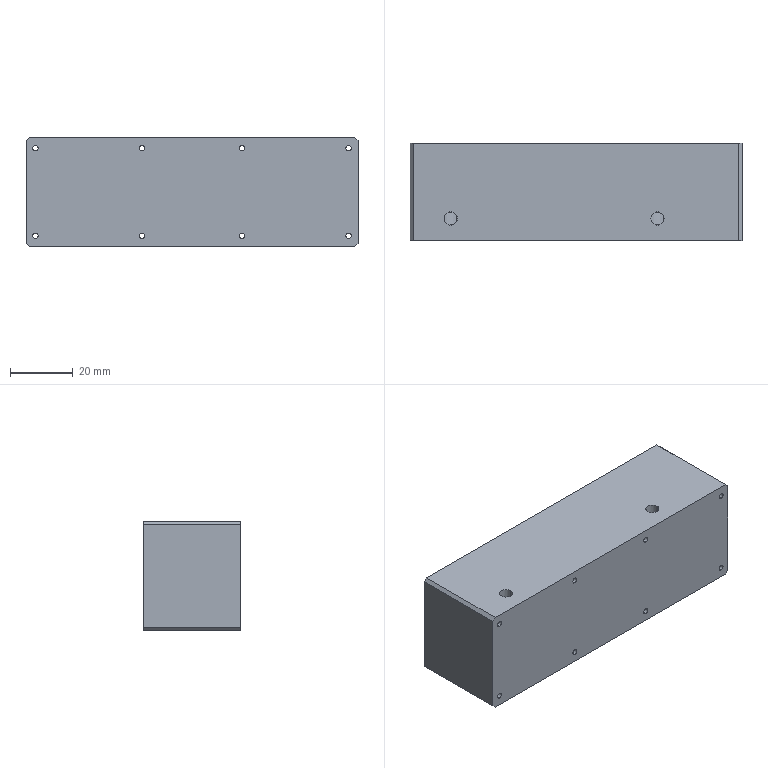Part | NX | features BREP 1 | 1 solid | 118 faces | box 106 x 31 x 35 mm | volume 87880 mm3 | cylinder 54 | cone 34 | plane 30 | commonest cylinder face diameters 10 x18 1.778 x16 3 x8 3.3 x8 4.2 x4